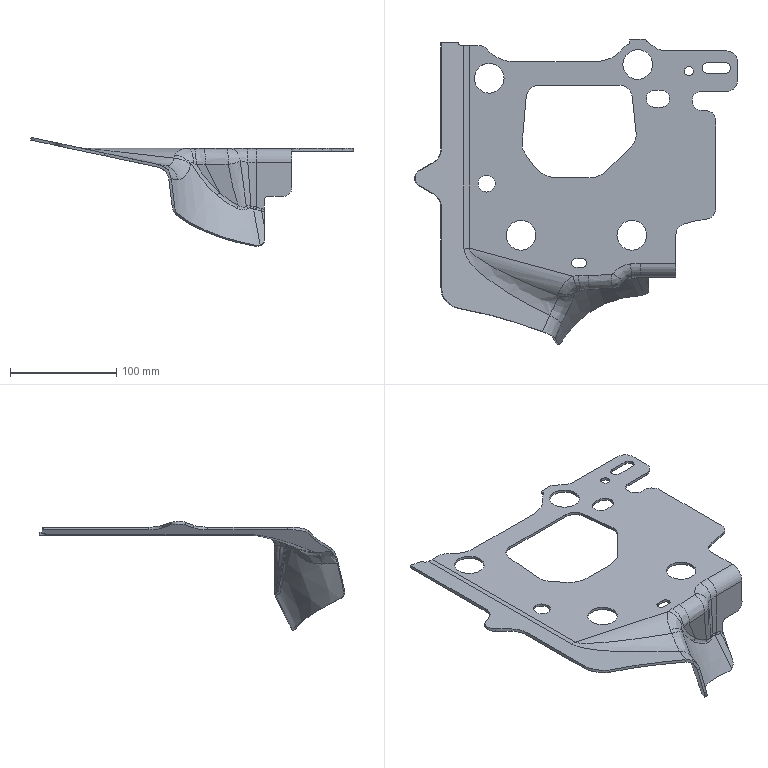Part | STEP file | lll_id174_x_t | 1 solid | 164 faces | box 304.48 x 287.796 x 102.85 mm | volume 141553 mm3 | spline 101 | plane 44 | cylinder 17 | torus 2 | commonest cylinder face diameters 1 x4 8.05 x2 55 x2 8.55 x1 21 x1 26 x1